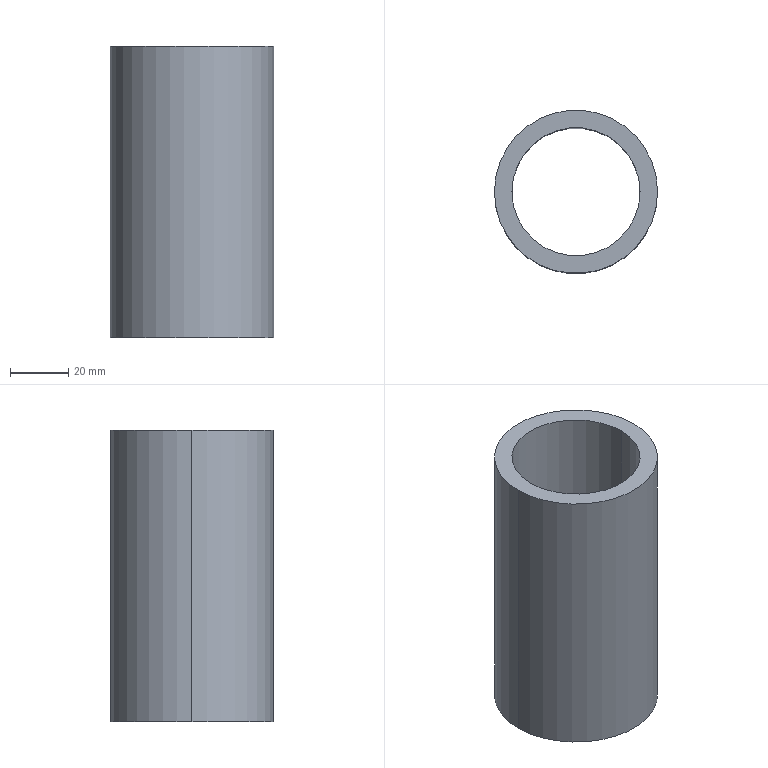Part | SolidWorks | features Extrusion 1 | 1 solid | 6 faces | box 56 x 56 x 100 mm | volume 94248 mm3 | cylinder 4 | plane 2 | commonest cylinder face diameters 44 x2 56 x2
STEP:
#1=CARTESIAN_POINT('',(-22.,0.,-50.));
#2=VERTEX_POINT('',#1);
#3=CARTESIAN_POINT('',(22.,0.,-50.));
#4=VERTEX_POINT('',#3);
#5=CARTESIAN_POINT('',(0.,0.,-50.));
#6=DIRECTION('',(0.,0.,1.));
#7=DIRECTION('',(1.,0.,0.));
#8=AXIS2_PLACEMENT_3D('',#5,#6,#7);
#9=CIRCLE('',#8,22.);
#10=EDGE_CURVE('',#2,#4,#9,.T.);
#11=ORIENTED_EDGE('',*,*,#10,.F.);
#12=CARTESIAN_POINT('',(-22.,0.,50.));
#13=VERTEX_POINT('',#12);
#14=CARTESIAN_POINT('',(-22.,0.,-50.));
#15=DIRECTION('',(0.,0.,1.));
#16=VECTOR('',#15,1000.);
#17=LINE('',#14,#16);
#18=EDGE_CURVE('',#2,#13,#17,.T.);
#19=ORIENTED_EDGE('',*,*,#18,.T.);
#20=CARTESIAN_POINT('',(22.,0.,50.));
#21=VERTEX_POINT('',#20);
#22=CARTESIAN_POINT('',(0.,0.,50.));
#23=DIRECTION('',(0.,0.,1.));
#24=DIRECTION('',(1.,0.,0.));
#25=AXIS2_PLACEMENT_3D('',#22,#23,#24);
#26=CIRCLE('',#25,22.);
#27=EDGE_CURVE('',#13,#21,#26,.T.);
#28=ORIENTED_EDGE('',*,*,#27,.T.);
#29=CARTESIAN_POINT('',(22.,0.,-50.));
#30=DIRECTION('',(0.,0.,1.));
#31=VECTOR('',#30,1000.);
#32=LINE('',#29,#31);
#33=EDGE_CURVE('',#4,#21,#32,.T.);
#34=ORIENTED_EDGE('',*,*,#33,.F.);
#35=EDGE_LOOP('',(#11,#19,#28,#34));
#36=FACE_OUTER_BOUND('',#35,.T.);
#37=CARTESIAN_POINT('',(0.,0.,-50.));
#38=DIRECTION('',(0.,0.,1.));
#39=DIRECTION('',(1.,0.,0.));
#40=AXIS2_PLACEMENT_3D('',#37,#38,#39);
#41=CYLINDRICAL_SURFACE('',#40,22.);
#42=ADVANCED_FACE('',(#36),#41,.F.);
#43=CARTESIAN_POINT('',(28.,0.,-50.));
#44=VERTEX_POINT('',#43);
#45=CARTESIAN_POINT('',(-28.,0.,-50.));
#46=VERTEX_POINT('',#45);
#47=CARTESIAN_POINT('',(0.,0.,-50.));
#48=DIRECTION('',(0.,0.,1.));
#49=DIRECTION('',(1.,0.,0.));
#50=AXIS2_PLACEMENT_3D('',#47,#48,#49);
#51=CIRCLE('',#50,28.);
#52=EDGE_CURVE('',#44,#46,#51,.T.);
#53=ORIENTED_EDGE('',*,*,#52,.T.);
#54=CARTESIAN_POINT('',(-28.,0.,50.));
#55=VERTEX_POINT('',#54);
#56=CARTESIAN_POINT('',(-28.,0.,-50.));
#57=DIRECTION('',(0.,0.,1.));
#58=VECTOR('',#57,1000.);
#59=LINE('',#56,#58);
#60=EDGE_CURVE('',#46,#55,#59,.T.);
#61=ORIENTED_EDGE('',*,*,#60,.T.);
#62=CARTESIAN_POINT('',(28.,0.,50.));
#63=VERTEX_POINT('',#62);
#64=CARTESIAN_POINT('',(0.,0.,50.));
#65=DIRECTION('',(0.,0.,1.));
#66=DIRECTION('',(1.,0.,0.));
#67=AXIS2_PLACEMENT_3D('',#64,#65,#66);
#68=CIRCLE('',#67,28.);
#69=EDGE_CURVE('',#63,#55,#68,.T.);
#70=ORIENTED_EDGE('',*,*,#69,.F.);
#71=CARTESIAN_POINT('',(28.,0.,-50.));
#72=DIRECTION('',(0.,0.,1.));
#73=VECTOR('',#72,1000.);
#74=LINE('',#71,#73);
#75=EDGE_CURVE('',#44,#63,#74,.T.);
#76=ORIENTED_EDGE('',*,*,#75,.F.);
#77=EDGE_LOOP('',(#53,#61,#70,#76));
#78=FACE_OUTER_BOUND('',#77,.T.);
#79=CARTESIAN_POINT('',(0.,0.,-50.));
#80=DIRECTION('',(0.,0.,1.));
#81=DIRECTION('',(1.,0.,0.));
#82=AXIS2_PLACEMENT_3D('',#79,#80,#81);
#83=CYLINDRICAL_SURFACE('',#82,28.);
#84=ADVANCED_FACE('',(#78),#83,.T.);
#85=ORIENTED_EDGE('',*,*,#60,.F.);
#86=CARTESIAN_POINT('',(0.,0.,-50.));
#87=DIRECTION('',(0.,0.,1.));
#88=DIRECTION('',(1.,0.,0.));
#89=AXIS2_PLACEMENT_3D('',#86,#87,#88);
#90=CIRCLE('',#89,28.);
#91=EDGE_CURVE('',#46,#44,#90,.T.);
#92=ORIENTED_EDGE('',*,*,#91,.T.);
#93=ORIENTED_EDGE('',*,*,#75,.T.);
#94=CARTESIAN_POINT('',(0.,0.,50.));
#95=DIRECTION('',(0.,0.,1.));
#96=DIRECTION('',(1.,0.,0.));
#97=AXIS2_PLACEMENT_3D('',#94,#95,#96);
#98=CIRCLE('',#97,28.);
#99=EDGE_CURVE('',#55,#63,#98,.T.);
#100=ORIENTED_EDGE('',*,*,#99,.F.);
#101=EDGE_LOOP('',(#85,#92,#93,#100));
#102=FACE_OUTER_BOUND('',#101,.T.);
#103=CARTESIAN_POINT('',(0.,0.,-50.));
#104=DIRECTION('',(0.,0.,1.));
#105=DIRECTION('',(1.,0.,0.));
#106=AXIS2_PLACEMENT_3D('',#103,#104,#105);
#107=CYLINDRICAL_SURFACE('',#106,28.);
#108=ADVANCED_FACE('',(#102),#107,.T.);
#109=CARTESIAN_POINT('',(0.,0.,-50.));
#110=DIRECTION('',(0.,0.,1.));
#111=DIRECTION('',(1.,0.,0.));
#112=AXIS2_PLACEMENT_3D('',#109,#110,#111);
#113=CIRCLE('',#112,22.);
#114=EDGE_CURVE('',#4,#2,#113,.T.);
#115=ORIENTED_EDGE('',*,*,#114,.T.);
#116=ORIENTED_EDGE('',*,*,#10,.T.);
#117=EDGE_LOOP('',(#115,#116));
#118=FACE_BOUND('',#117,.T.);
#119=ORIENTED_EDGE('',*,*,#52,.F.);
#120=ORIENTED_EDGE('',*,*,#91,.F.);
#121=EDGE_LOOP('',(#119,#120));
#122=FACE_OUTER_BOUND('',#121,.T.);
#123=CARTESIAN_POINT('',(0.,0.,-50.));
#124=DIRECTION('',(0.,0.,1.));
#125=DIRECTION('',(1.,0.,0.));
#126=AXIS2_PLACEMENT_3D('',#123,#124,#125);
#127=PLANE('',#126);
#128=ADVANCED_FACE('',(#118,#122),#127,.F.);
#129=CARTESIAN_POINT('',(0.,0.,50.));
#130=DIRECTION('',(0.,0.,1.));
#131=DIRECTION('',(1.,0.,0.));
#132=AXIS2_PLACEMENT_3D('',#129,#130,#131);
#133=CIRCLE('',#132,22.);
#134=EDGE_CURVE('',#21,#13,#133,.T.);
#135=ORIENTED_EDGE('',*,*,#134,.F.);
#136=ORIENTED_EDGE('',*,*,#27,.F.);
#137=EDGE_LOOP('',(#135,#136));
#138=FACE_BOUND('',#137,.T.);
#139=ORIENTED_EDGE('',*,*,#69,.T.);
#140=ORIENTED_EDGE('',*,*,#99,.T.);
#141=EDGE_LOOP('',(#139,#140));
#142=FACE_OUTER_BOUND('',#141,.T.);
#143=CARTESIAN_POINT('',(0.,0.,50.));
#144=DIRECTION('',(0.,0.,1.));
#145=DIRECTION('',(1.,0.,0.));
#146=AXIS2_PLACEMENT_3D('',#143,#144,#145);
#147=PLANE('',#146);
#148=ADVANCED_FACE('',(#138,#142),#147,.T.);
#149=ORIENTED_EDGE('',*,*,#18,.F.);
#150=ORIENTED_EDGE('',*,*,#114,.F.);
#151=ORIENTED_EDGE('',*,*,#33,.T.);
#152=ORIENTED_EDGE('',*,*,#134,.T.);
#153=EDGE_LOOP('',(#149,#150,#151,#152));
#154=FACE_OUTER_BOUND('',#153,.T.);
#155=CARTESIAN_POINT('',(0.,0.,-50.));
#156=DIRECTION('',(0.,0.,1.));
#157=DIRECTION('',(1.,0.,0.));
#158=AXIS2_PLACEMENT_3D('',#155,#156,#157);
#159=CYLINDRICAL_SURFACE('',#158,22.);
#160=ADVANCED_FACE('',(#154),#159,.F.);
#161=CLOSED_SHELL('',(#42,#84,#108,#128,#148,#160));
#162=MANIFOLD_SOLID_BREP('',#161);
#163=CARTESIAN_POINT('',(0.,0.,0.));
#164=DIRECTION('',(0.,0.,1.));
#165=DIRECTION('',(1.,0.,0.));
#166=AXIS2_PLACEMENT_3D('',#163,#164,#165);
#167=(LENGTH_UNIT()NAMED_UNIT(*)SI_UNIT(.MILLI.,.METRE.));
#168=UNCERTAINTY_MEASURE_WITH_UNIT(LENGTH_MEASURE(0.00001),#167,'','');
#169=(NAMED_UNIT(*)PLANE_ANGLE_UNIT()SI_UNIT($,.RADIAN.));
#170=(NAMED_UNIT(*)SI_UNIT($,.STERADIAN.)SOLID_ANGLE_UNIT());
#171=(GEOMETRIC_REPRESENTATION_CONTEXT(3)GLOBAL_UNCERTAINTY_ASSIGNED_CONTEXT((#168))GLOBAL_UNIT_ASSIGNED_CONTEXT((#167,#169,#170))REPRESENTATION_CONTEXT('',''));
#172=ADVANCED_BREP_SHAPE_REPRESENTATION('',(#162,#166),#171);